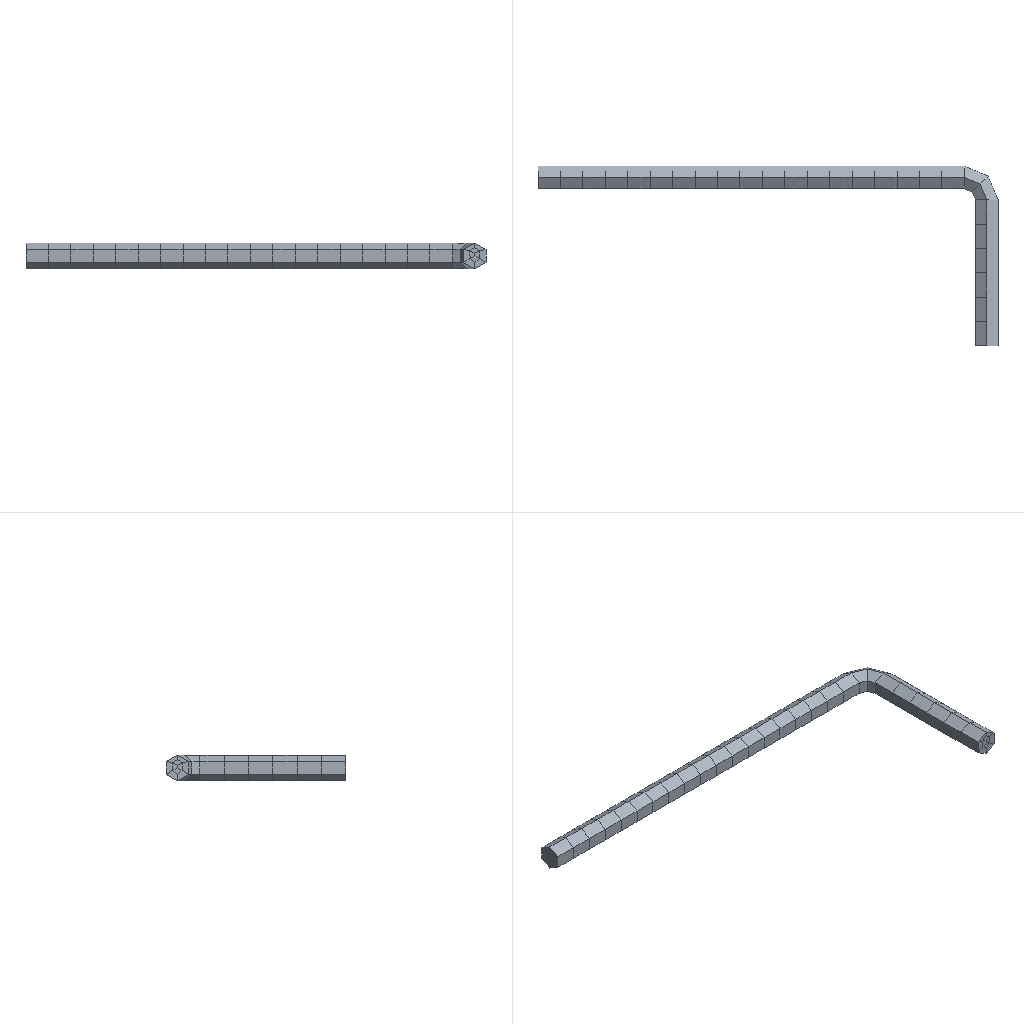Simulation study | ansys workbench
Ansys APDL input file, long lists of numbers shortened:
/batch
/config,noeldb,1     ! force off writing results to database
*get,_wallstrt,active,,time,wall
! ANSYS input file written by Workbench version 2022 R1
! File used for geometry attach:
/title,wbnew--____ (A5)
! ****** Begin Custom Load Command Snippet ******
/COM, ACT Extensions:
/COM,     LSDYNA, 2021.1
/COM,
! ****** End   Custom Load Command Snippet ******
*DIM,_wb_ProjectScratch_dir,string,248
_wb_ProjectScratch_dir(1) = ''
*DIM,_wb_SolverFiles_dir,string,248
_wb_SolverFiles_dir(1) = ''
*DIM,_wb_userfiles_dir,string,248
_wb_userfiles_dir(1) = ''
/com,--- Data in consistent NMM units. See Solving Units in the help system for more information.
/units,MPA
/nopr
/wb,file,start              !  signify a WB generated input file
/prep7
! Turn off shape checking because checks already performed inside WB mesher.
! See help system for more information.
SHPP,OFF,,NOWARN
/nolist
etcon,set             ! allow ANSYS to choose best KEYOP's for 180x elements, resets any applicable keyopt to MAPDL defaults
/com,*********** Nodes for the whole assembly ***********
nblock,3,,1555
(1i9,3e20.9e3)
        1     1.000000000E+01     4.526588428E-02     2.653613818E-02
! (1413 more lines like these left out)
-1
/wb,elem,start            !  set before creation of elements
/com,*********** Elements for Body 1 "_____-FreeParts|__1" ***********
et,1,186
keyo,1,2,1          ! set full integration on SOLID186
eblock,19,solid,,270
(19i9)
        1        1        1        1        0        0        0        0       20        0        1        1        3        5        4      216      214      212      213
! (539 more lines like these left out)
-1
/wb,elem,end               !  done creating elements
/com,*********** Send User Defined Coordinate System(s) ***********
csys,0
toffst,273.15,  ! Temperature offset from absolute zero
/com,*********** Set Reference Temperature ***********
tref,22.
/wb,mat,start              !  starting to send materials
/com,*********** Send Materials ***********
Temperature = 'TEMP' ! Temperature
MP,DENS,1,7.85e-09,	! tonne mm^-3
MP,ALPX,1,1.2e-05,	! C^-1
MP,C,1,434000000,	! mm^2 s^-2 C^-1
MP,KXX,1,60.5,	! tonne mm s^-3 C^-1
MP,RSVX,1,0.00017,	! ohm mm
MP,EX,1,200000,	! tonne s^-2 mm^-1
MP,NUXY,1,0.3,
MP,MURX,1,10000,
/wb,mat,end                !  done sending materials
!************************* Model Summary ********************
!_____-FreeParts|__1,	结构钢,	matid,	1
!************************* End Model Summary ********************
! get the diagonal of the bounding box. Needed later for other things
*get,_xmin,node,,mnloc,x
*get,_ymin,node,,mnloc,y
*get,_zmin,node,,mnloc,z
*get,_xmax,node,,mxloc,x
*get,_ymax,node,,mxloc,y
*get,_zmax,node,,mxloc,z
_ASMDIAG=(_xmax-_xmin)*(_xmax-_xmin)+(_ymax-_ymin)*(_ymax-_ymin)+(_zmax-_zmin)*(_zmax-_zmin)
_ASMDIAG=SQRT(_ASMDIAG)
/wb,contact,start          !  starting to send contact
/wb,contact,end            !  done creating contacts
/golist
/wb,load,start             !  starting to send loads
/com,*********** Fixed Supports ***********
CMBLOCK,_FIXEDSU,NODE,       37
(8i10)
       217       218       219       220       221       222       223       224
       225       226       227       228       229       230      1068      1069
      1070      1071      1072      1073      1074      1075      1076      1077
      1078      1079      1080      1081      1082      1083      1084      1085
      1086      1088      1090      1092      1094
cmsel,s,_FIXEDSU
d,all,all
nsel,all
/com,*********** Define Force Using Surface Effect Elements ***********
local,12,0,0.,0.,0.,0.,0.,0.
csys,0
et,2,154
eblock,10,,,38
(15i9)
      453        2        2        2       12      316      315      334      335     1283     1284     1320     1285
! (37 more lines like these left out)
-1
esel,s,type,,2
keyop,2,2,1                ! Apply load in local coordinate system
keyop,2,7,1                ! Use original area so load is constant in large deformation
esel,all
/com,*********** Define Force Using Surface Effect Elements ***********
local,13,0,0.,0.,0.,0.,0.,0.
csys,0
et,3,154
eblock,10,,,19
(15i9)
      491        3        3        3       13      354      353      372      373     1357     1358     1394     1359
! (18 more lines like these left out)
-1
esel,s,type,,3
keyop,3,2,1                ! Apply load in local coordinate system
keyop,3,7,1                ! Use original area so load is constant in large deformation
esel,all
/gst,on,on
fini
*get,_numnode,node,0,count
*get,_numelem,elem,0,count
*get, _MAXELEMNUM, elem, 0, NUM, MAX
*get, _MAXNODENUM, node, 0, NUM, MAX
*get, _MAXELEMTYPE, etyp, 0, NUM, MAX
*get, _MAXREALCONST, real, 0, NUM, MAX
/go
/wb,load,end               !  done creating loads
/com,--- Number of total nodes = %_numnode%
/com,--- Number of contact elements = 57
/com,--- Number of spring elements = 0
/com,--- Number of bearing elements = 0
/com,--- Number of solid elements = 270
/com,--- Number of condensed parts = 0
/com,--- Number of total elements = %_numelem%
*get,_wallbsol,active,,time,wall
/com,****************************************************************************
/com,*************************    SOLUTION       ********************************
/com,****************************************************************************
/solu
antype,0                   ! static analysis
_thickRatio=  1     ! Ratio of thick parts in the model
eqsl,pcg,1e-8,,,,,,1
cntr,print,1               ! print out contact info and also make no initial contact an error
dmpoption,emat,no             ! Don't combine emat file for DANSYS
dmpoption,esav,no             ! Don't combine esav file for DANSYS
nldiag,cont,iter           ! print out contact info each equilibrium iteration
rescontrol,,none                 ! Do not keep any restart files
/com,****************************************************
/com,******************* SOLVE FOR LS 1 OF 1 ****************
esel,s,type,,2
nsle
sfe,all,1,pres,1,0.
sfe,all,2,pres,1,0.
sfe,all,3,pres,1,-4.55802844097109e-002
esel,s,type,,3
nsle
sfe,all,1,pres,1,0.
sfe,all,2,pres,1,-1.82321137638844e-002
sfe,all,3,pres,1,-6.02588145656589e-017
nsel,all
esel,all
/nopr
/gopr
nsub,1,1,1
time,1.
outres,erase
outres,all,none
outres,nsol,all,
outres,rsol,all
outres,eangl,all
outres,etmp,all
outres,veng,all
outres,strs,all,
outres,epel,all,
outres,eppl,all,
outres,cont,all,
! *********** WB SOLVE COMMAND ***********
! check interactive state
*get,ANSINTER_,active,,int
*if,ANSINTER_,ne,0,then
/eof
*endif
solve
/com *************** Write FE CONNECTORS *********
CEWRITE,file,ce,,INTE
/com,****************************************************
/com,*************** FINISHED SOLVE FOR LS 1 *************
*get,_wallasol,active,,time,wall
/nopr
*get,_numnode,node,0,count
*get,_numelem,elem,0,count
*get, _MAXELEMNUM, elem, 0, NUM, MAX
*get, _MAXNODENUM, node, 0, NUM, MAX,,,INTERNAL
*get, _MAXELEMTYPE, etyp, 0, NUM, MAX
*get, _MAXREALCONST, real, 0, NUM, MAX
/gopr
*get,_PCGITER,active,,solu,cgiter
/post1
xmlo,ENCODING,ISO-8859-1
xmlo,parm
/xml,parm,xml
fini
/gopr
*get,_walldone,active,,time,wall
_preptime=(_wallbsol-_wallstrt)*3600
_solvtime=(_wallasol-_wallbsol)*3600
_posttime=(_walldone-_wallasol)*3600
_totaltim=(_walldone-_wallstrt)*3600
*get,_dlbratio,active,0,solu,dlbr
*get,_combtime,active,0,solu,comb
*get,_ssmode,active,0,solu,ssmm
*get,_ndofs,active,0,solu,ndof
*get,_sol_end_time,active,0,set,time
*if,_sol_end_time,eq,1.,then
/fclean				!clean distributed files
*endif
/com,--- Total number of nodes = %_numnode%
/com,--- Total number of elements = %_numelem%
/com,--- Element load balance ratio = %_dlbratio%
/com,--- Time to combine distributed files = %_combtime%
/com,--- Sparse memory mode = %_ssmode%
/com,--- Number of DOF = %_ndofs%
/wb,file,end               ! done with WB generated input